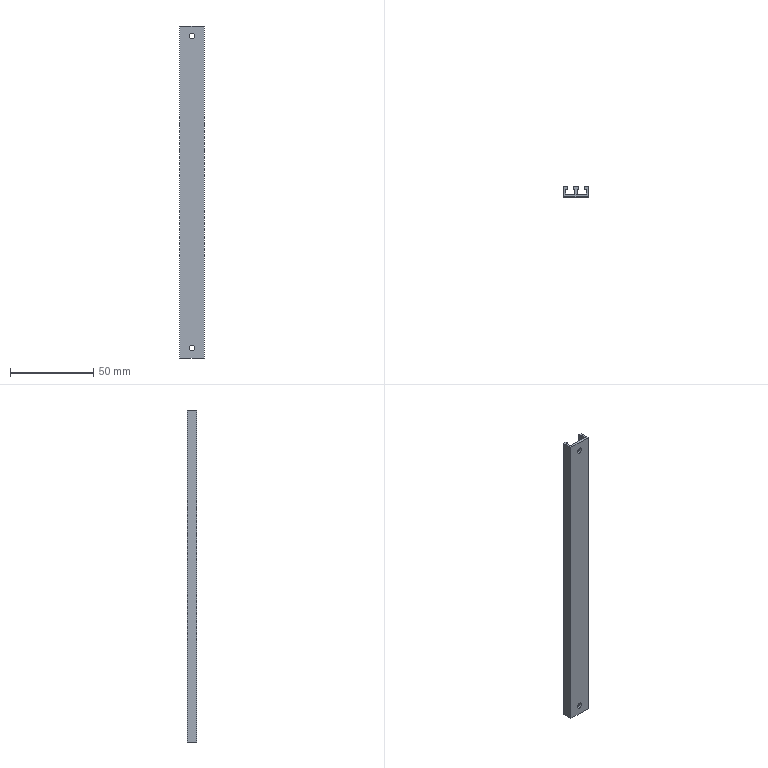Part | STEP file | 10-16 camera shaft sensor mounting strip | 1 solid | 39 faces | box 15 x 6 x 200 mm | volume 9017 mm3 | plane 23 | cylinder 16 | commonest cylinder face diameters 0.4 x12 3.5 x4
STEP:
#1=CARTESIAN_POINT('',(7.5,1.5,-292.25));
#2=VERTEX_POINT('',#1);
#3=CARTESIAN_POINT('',(7.5,1.5,-295.75));
#4=VERTEX_POINT('',#3);
#5=CARTESIAN_POINT('',(7.5,1.5,-294.));
#6=DIRECTION('',(0.,-1.,0.));
#7=DIRECTION('',(1.,0.,0.));
#8=AXIS2_PLACEMENT_3D('',#5,#6,#7);
#9=CIRCLE('',#8,1.75);
#10=EDGE_CURVE('',#2,#4,#9,.T.);
#11=ORIENTED_EDGE('',*,*,#10,.F.);
#12=CARTESIAN_POINT('',(7.5,0.,-292.25));
#13=VERTEX_POINT('',#12);
#14=CARTESIAN_POINT('',(7.5,0.,-292.25));
#15=DIRECTION('',(0.,-1.,0.));
#16=VECTOR('',#15,1000.);
#17=LINE('',#14,#16);
#18=EDGE_CURVE('',#2,#13,#17,.T.);
#19=ORIENTED_EDGE('',*,*,#18,.T.);
#20=CARTESIAN_POINT('',(7.5,0.,-295.75));
#21=VERTEX_POINT('',#20);
#22=CARTESIAN_POINT('',(7.5,0.,-294.));
#23=DIRECTION('',(0.,-1.,0.));
#24=DIRECTION('',(0.,0.,-1.));
#25=AXIS2_PLACEMENT_3D('',#22,#23,#24);
#26=CIRCLE('',#25,1.75);
#27=EDGE_CURVE('',#13,#21,#26,.T.);
#28=ORIENTED_EDGE('',*,*,#27,.T.);
#29=CARTESIAN_POINT('',(7.5,0.,-295.75));
#30=DIRECTION('',(0.,-1.,0.));
#31=VECTOR('',#30,1000.);
#32=LINE('',#29,#31);
#33=EDGE_CURVE('',#4,#21,#32,.T.);
#34=ORIENTED_EDGE('',*,*,#33,.F.);
#35=EDGE_LOOP('',(#11,#19,#28,#34));
#36=FACE_OUTER_BOUND('',#35,.T.);
#37=CARTESIAN_POINT('',(7.5,0.,-294.));
#38=DIRECTION('',(0.,-1.,0.));
#39=DIRECTION('',(0.,0.,-1.));
#40=AXIS2_PLACEMENT_3D('',#37,#38,#39);
#41=CYLINDRICAL_SURFACE('',#40,1.75);
#42=ADVANCED_FACE('',(#36),#41,.F.);
#43=CARTESIAN_POINT('',(7.5,1.5,-104.25));
#44=VERTEX_POINT('',#43);
#45=CARTESIAN_POINT('',(7.5,1.5,-107.75));
#46=VERTEX_POINT('',#45);
#47=CARTESIAN_POINT('',(7.5,1.5,-106.));
#48=DIRECTION('',(0.,-1.,0.));
#49=DIRECTION('',(1.,0.,0.));
#50=AXIS2_PLACEMENT_3D('',#47,#48,#49);
#51=CIRCLE('',#50,1.75);
#52=EDGE_CURVE('',#44,#46,#51,.T.);
#53=ORIENTED_EDGE('',*,*,#52,.F.);
#54=CARTESIAN_POINT('',(7.5,0.,-104.25));
#55=VERTEX_POINT('',#54);
#56=CARTESIAN_POINT('',(7.5,0.,-104.25));
#57=DIRECTION('',(0.,-1.,0.));
#58=VECTOR('',#57,1000.);
#59=LINE('',#56,#58);
#60=EDGE_CURVE('',#44,#55,#59,.T.);
#61=ORIENTED_EDGE('',*,*,#60,.T.);
#62=CARTESIAN_POINT('',(7.5,0.,-107.75));
#63=VERTEX_POINT('',#62);
#64=CARTESIAN_POINT('',(7.5,0.,-106.));
#65=DIRECTION('',(0.,-1.,0.));
#66=DIRECTION('',(0.,0.,-1.));
#67=AXIS2_PLACEMENT_3D('',#64,#65,#66);
#68=CIRCLE('',#67,1.75);
#69=EDGE_CURVE('',#55,#63,#68,.T.);
#70=ORIENTED_EDGE('',*,*,#69,.T.);
#71=CARTESIAN_POINT('',(7.5,0.,-107.75));
#72=DIRECTION('',(0.,-1.,0.));
#73=VECTOR('',#72,1000.);
#74=LINE('',#71,#73);
#75=EDGE_CURVE('',#46,#63,#74,.T.);
#76=ORIENTED_EDGE('',*,*,#75,.F.);
#77=EDGE_LOOP('',(#53,#61,#70,#76));
#78=FACE_OUTER_BOUND('',#77,.T.);
#79=CARTESIAN_POINT('',(7.5,0.,-106.));
#80=DIRECTION('',(0.,-1.,0.));
#81=DIRECTION('',(0.,0.,-1.));
#82=AXIS2_PLACEMENT_3D('',#79,#80,#81);
#83=CYLINDRICAL_SURFACE('',#82,1.75);
#84=ADVANCED_FACE('',(#78),#83,.F.);
#85=CARTESIAN_POINT('',(8.25,4.5,-112.));
#86=VERTEX_POINT('',#85);
#87=CARTESIAN_POINT('',(8.25,4.5,-288.));
#88=VERTEX_POINT('',#87);
#89=CARTESIAN_POINT('',(8.25,4.5,-288.));
#90=DIRECTION('',(0.,0.,-1.));
#91=VECTOR('',#90,1000.);
#92=LINE('',#89,#91);
#93=EDGE_CURVE('',#86,#88,#92,.T.);
#94=ORIENTED_EDGE('',*,*,#93,.F.);
#95=CARTESIAN_POINT('',(8.25,1.5,-112.));
#96=VERTEX_POINT('',#95);
#97=CARTESIAN_POINT('',(8.25,6.,-112.));
#98=DIRECTION('',(0.,-1.,0.));
#99=VECTOR('',#98,1000.);
#100=LINE('',#97,#99);
#101=EDGE_CURVE('',#86,#96,#100,.T.);
#102=ORIENTED_EDGE('',*,*,#101,.T.);
#103=CARTESIAN_POINT('',(8.25,1.5,-288.));
#104=VERTEX_POINT('',#103);
#105=CARTESIAN_POINT('',(8.25,1.5,-288.));
#106=DIRECTION('',(0.,0.,-1.));
#107=VECTOR('',#106,1000.);
#108=LINE('',#105,#107);
#109=EDGE_CURVE('',#96,#104,#108,.T.);
#110=ORIENTED_EDGE('',*,*,#109,.T.);
#111=CARTESIAN_POINT('',(8.25,6.,-288.));
#112=DIRECTION('',(0.,-1.,0.));
#113=VECTOR('',#112,1000.);
#114=LINE('',#111,#113);
#115=EDGE_CURVE('',#88,#104,#114,.T.);
#116=ORIENTED_EDGE('',*,*,#115,.F.);
#117=EDGE_LOOP('',(#94,#102,#110,#116));
#118=FACE_OUTER_BOUND('',#117,.T.);
#119=CARTESIAN_POINT('',(8.25,6.,-288.));
#120=DIRECTION('',(-1.,0.,0.));
#121=DIRECTION('',(0.,-1.,0.));
#122=AXIS2_PLACEMENT_3D('',#119,#120,#121);
#123=PLANE('',#122);
#124=ADVANCED_FACE('',(#118),#123,.F.);
#125=CARTESIAN_POINT('',(6.75,4.5,-288.));
#126=VERTEX_POINT('',#125);
#127=CARTESIAN_POINT('',(6.75,4.5,-112.));
#128=VERTEX_POINT('',#127);
#129=CARTESIAN_POINT('',(6.75,4.5,-112.));
#130=DIRECTION('',(0.,0.,1.));
#131=VECTOR('',#130,1000.);
#132=LINE('',#129,#131);
#133=EDGE_CURVE('',#126,#128,#132,.T.);
#134=ORIENTED_EDGE('',*,*,#133,.F.);
#135=CARTESIAN_POINT('',(6.75,1.5,-288.));
#136=VERTEX_POINT('',#135);
#137=CARTESIAN_POINT('',(6.75,6.,-288.));
#138=DIRECTION('',(0.,-1.,0.));
#139=VECTOR('',#138,1000.);
#140=LINE('',#137,#139);
#141=EDGE_CURVE('',#126,#136,#140,.T.);
#142=ORIENTED_EDGE('',*,*,#141,.T.);
#143=CARTESIAN_POINT('',(6.75,1.5,-112.));
#144=VERTEX_POINT('',#143);
#145=CARTESIAN_POINT('',(6.75,1.5,-112.));
#146=DIRECTION('',(0.,0.,1.));
#147=VECTOR('',#146,1000.);
#148=LINE('',#145,#147);
#149=EDGE_CURVE('',#136,#144,#148,.T.);
#150=ORIENTED_EDGE('',*,*,#149,.T.);
#151=CARTESIAN_POINT('',(6.75,6.,-112.));
#152=DIRECTION('',(0.,-1.,0.));
#153=VECTOR('',#152,1000.);
#154=LINE('',#151,#153);
#155=EDGE_CURVE('',#128,#144,#154,.T.);
#156=ORIENTED_EDGE('',*,*,#155,.F.);
#157=EDGE_LOOP('',(#134,#142,#150,#156));
#158=FACE_OUTER_BOUND('',#157,.T.);
#159=CARTESIAN_POINT('',(6.75,6.,-112.));
#160=DIRECTION('',(1.,0.,0.));
#161=DIRECTION('',(0.,1.,0.));
#162=AXIS2_PLACEMENT_3D('',#159,#160,#161);
#163=PLANE('',#162);
#164=ADVANCED_FACE('',(#158),#163,.F.);
#165=CARTESIAN_POINT('',(7.5,1.5,-294.));
#166=DIRECTION('',(0.,-1.,0.));
#167=DIRECTION('',(1.,0.,0.));
#168=AXIS2_PLACEMENT_3D('',#165,#166,#167);
#169=CIRCLE('',#168,1.75);
#170=EDGE_CURVE('',#4,#2,#169,.T.);
#171=ORIENTED_EDGE('',*,*,#170,.T.);
#172=ORIENTED_EDGE('',*,*,#10,.T.);
#173=EDGE_LOOP('',(#171,#172));
#174=FACE_BOUND('',#173,.T.);
#175=CARTESIAN_POINT('',(7.5,1.5,-106.));
#176=DIRECTION('',(0.,-1.,0.));
#177=DIRECTION('',(1.,0.,0.));
#178=AXIS2_PLACEMENT_3D('',#175,#176,#177);
#179=CIRCLE('',#178,1.75);
#180=EDGE_CURVE('',#46,#44,#179,.T.);
#181=ORIENTED_EDGE('',*,*,#180,.T.);
#182=ORIENTED_EDGE('',*,*,#52,.T.);
#183=EDGE_LOOP('',(#181,#182));
#184=FACE_BOUND('',#183,.T.);
#185=CARTESIAN_POINT('',(1.25,1.5,-100.));
#186=VERTEX_POINT('',#185);
#187=CARTESIAN_POINT('',(13.75,1.5,-100.));
#188=VERTEX_POINT('',#187);
#189=CARTESIAN_POINT('',(1.25,1.5,-100.));
#190=DIRECTION('',(1.,0.,0.));
#191=VECTOR('',#190,1000.);
#192=LINE('',#189,#191);
#193=EDGE_CURVE('',#186,#188,#192,.T.);
#194=ORIENTED_EDGE('',*,*,#193,.T.);
#195=CARTESIAN_POINT('',(13.75,1.5,-300.));
#196=VERTEX_POINT('',#195);
#197=CARTESIAN_POINT('',(13.75,1.5,-300.));
#198=DIRECTION('',(0.,0.,1.));
#199=VECTOR('',#198,1000.);
#200=LINE('',#197,#199);
#201=EDGE_CURVE('',#196,#188,#200,.T.);
#202=ORIENTED_EDGE('',*,*,#201,.F.);
#203=CARTESIAN_POINT('',(1.25,1.5,-300.));
#204=VERTEX_POINT('',#203);
#205=CARTESIAN_POINT('',(1.25,1.5,-300.));
#206=DIRECTION('',(1.,0.,0.));
#207=VECTOR('',#206,1000.);
#208=LINE('',#205,#207);
#209=EDGE_CURVE('',#204,#196,#208,.T.);
#210=ORIENTED_EDGE('',*,*,#209,.F.);
#211=CARTESIAN_POINT('',(1.25,1.5,-300.));
#212=DIRECTION('',(0.,0.,1.));
#213=VECTOR('',#212,1000.);
#214=LINE('',#211,#213);
#215=EDGE_CURVE('',#204,#186,#214,.T.);
#216=ORIENTED_EDGE('',*,*,#215,.T.);
#217=EDGE_LOOP('',(#194,#202,#210,#216));
#218=FACE_OUTER_BOUND('',#217,.T.);
#219=CARTESIAN_POINT('',(6.75,1.5,-288.));
#220=DIRECTION('',(-1.,0.,0.));
#221=VECTOR('',#220,1000.);
#222=LINE('',#219,#221);
#223=EDGE_CURVE('',#104,#136,#222,.T.);
#224=ORIENTED_EDGE('',*,*,#223,.F.);
#225=ORIENTED_EDGE('',*,*,#109,.F.);
#226=CARTESIAN_POINT('',(8.25,1.5,-112.));
#227=DIRECTION('',(1.,0.,0.));
#228=VECTOR('',#227,1000.);
#229=LINE('',#226,#228);
#230=EDGE_CURVE('',#144,#96,#229,.T.);
#231=ORIENTED_EDGE('',*,*,#230,.F.);
#232=ORIENTED_EDGE('',*,*,#149,.F.);
#233=EDGE_LOOP('',(#224,#225,#231,#232));
#234=FACE_BOUND('',#233,.T.);
#235=CARTESIAN_POINT('',(1.25,1.5,-300.));
#236=DIRECTION('',(0.,-1.,0.));
#237=DIRECTION('',(1.,0.,0.));
#238=AXIS2_PLACEMENT_3D('',#235,#236,#237);
#239=PLANE('',#238);
#240=ADVANCED_FACE('',(#174,#184,#218,#234),#239,.F.);
#241=CARTESIAN_POINT('',(12.95,6.,-100.));
#242=VERTEX_POINT('',#241);
#243=CARTESIAN_POINT('',(14.8,6.,-100.));
#244=VERTEX_POINT('',#243);
#245=CARTESIAN_POINT('',(0.,6.,-100.));
#246=DIRECTION('',(1.,0.,0.));
#247=VECTOR('',#246,1000.);
#248=LINE('',#245,#247);
#249=EDGE_CURVE('',#242,#244,#248,.T.);
#250=ORIENTED_EDGE('',*,*,#249,.T.);
#251=CARTESIAN_POINT('',(14.8,6.,-300.));
#252=VERTEX_POINT('',#251);
#253=CARTESIAN_POINT('',(14.8,6.,-100.));
#254=DIRECTION('',(0.,0.,-1.));
#255=VECTOR('',#254,1000.);
#256=LINE('',#253,#255);
#257=EDGE_CURVE('',#244,#252,#256,.T.);
#258=ORIENTED_EDGE('',*,*,#257,.T.);
#259=CARTESIAN_POINT('',(12.95,6.,-300.));
#260=VERTEX_POINT('',#259);
#261=CARTESIAN_POINT('',(15.,6.,-300.));
#262=DIRECTION('',(-1.,0.,0.));
#263=VECTOR('',#262,1000.);
#264=LINE('',#261,#263);
#265=EDGE_CURVE('',#252,#260,#264,.T.);
#266=ORIENTED_EDGE('',*,*,#265,.T.);
#267=CARTESIAN_POINT('',(12.95,6.,-100.));
#268=DIRECTION('',(0.,0.,1.));
#269=VECTOR('',#268,1000.);
#270=LINE('',#267,#269);
#271=EDGE_CURVE('',#260,#242,#270,.T.);
#272=ORIENTED_EDGE('',*,*,#271,.T.);
#273=EDGE_LOOP('',(#250,#258,#266,#272));
#274=FACE_OUTER_BOUND('',#273,.T.);
#275=CARTESIAN_POINT('',(0.,6.,-100.));
#276=DIRECTION('',(0.,1.,0.));
#277=DIRECTION('',(0.,0.,1.));
#278=AXIS2_PLACEMENT_3D('',#275,#276,#277);
#279=PLANE('',#278);
#280=ADVANCED_FACE('',(#274),#279,.T.);
#281=CARTESIAN_POINT('',(0.,0.2,-100.));
#282=VERTEX_POINT('',#281);
#283=CARTESIAN_POINT('',(0.,5.8,-100.));
#284=VERTEX_POINT('',#283);
#285=CARTESIAN_POINT('',(0.,0.,-100.));
#286=DIRECTION('',(0.,1.,0.));
#287=VECTOR('',#286,1000.);
#288=LINE('',#285,#287);
#289=EDGE_CURVE('',#282,#284,#288,.T.);
#290=ORIENTED_EDGE('',*,*,#289,.T.);
#291=CARTESIAN_POINT('',(0.,5.8,-300.));
#292=VERTEX_POINT('',#291);
#293=CARTESIAN_POINT('',(0.,5.8,-300.));
#294=DIRECTION('',(0.,0.,-1.));
#295=VECTOR('',#294,1000.);
#296=LINE('',#293,#295);
#297=EDGE_CURVE('',#284,#292,#296,.T.);
#298=ORIENTED_EDGE('',*,*,#297,.T.);
#299=CARTESIAN_POINT('',(0.,0.2,-300.));
#300=VERTEX_POINT('',#299);
#301=CARTESIAN_POINT('',(0.,0.,-300.));
#302=DIRECTION('',(0.,1.,0.));
#303=VECTOR('',#302,1000.);
#304=LINE('',#301,#303);
#305=EDGE_CURVE('',#300,#292,#304,.T.);
#306=ORIENTED_EDGE('',*,*,#305,.F.);
#307=CARTESIAN_POINT('',(0.,0.2,-100.));
#308=DIRECTION('',(0.,0.,1.));
#309=VECTOR('',#308,1000.);
#310=LINE('',#307,#309);
#311=EDGE_CURVE('',#300,#282,#310,.T.);
#312=ORIENTED_EDGE('',*,*,#311,.T.);
#313=EDGE_LOOP('',(#290,#298,#306,#312));
#314=FACE_OUTER_BOUND('',#313,.T.);
#315=CARTESIAN_POINT('',(0.,0.,-300.));
#316=DIRECTION('',(-1.,0.,0.));
#317=DIRECTION('',(0.,0.,1.));
#318=AXIS2_PLACEMENT_3D('',#315,#316,#317);
#319=PLANE('',#318);
#320=ADVANCED_FACE('',(#314),#319,.T.);
#321=ORIENTED_EDGE('',*,*,#305,.T.);
#322=CARTESIAN_POINT('',(0.2,6.,-300.));
#323=VERTEX_POINT('',#322);
#324=CARTESIAN_POINT('',(0.2,5.8,-300.));
#325=DIRECTION('',(0.,0.,-1.));
#326=DIRECTION('',(-1.,0.,0.));
#327=AXIS2_PLACEMENT_3D('',#324,#325,#326);
#328=CIRCLE('',#327,0.2);
#329=EDGE_CURVE('',#292,#323,#328,.T.);
#330=ORIENTED_EDGE('',*,*,#329,.T.);
#331=CARTESIAN_POINT('',(2.05,6.,-300.));
#332=VERTEX_POINT('',#331);
#333=CARTESIAN_POINT('',(15.,6.,-300.));
#334=DIRECTION('',(-1.,0.,0.));
#335=VECTOR('',#334,1000.);
#336=LINE('',#333,#335);
#337=EDGE_CURVE('',#332,#323,#336,.T.);
#338=ORIENTED_EDGE('',*,*,#337,.F.);
#339=CARTESIAN_POINT('',(2.25,5.8,-300.));
#340=VERTEX_POINT('',#339);
#341=CARTESIAN_POINT('',(2.05,5.8,-300.));
#342=DIRECTION('',(0.,0.,-1.));
#343=DIRECTION('',(-1.,0.,0.));
#344=AXIS2_PLACEMENT_3D('',#341,#342,#343);
#345=CIRCLE('',#344,0.2);
#346=EDGE_CURVE('',#332,#340,#345,.T.);
#347=ORIENTED_EDGE('',*,*,#346,.T.);
#348=CARTESIAN_POINT('',(2.25,4.7,-300.));
#349=VERTEX_POINT('',#348);
#350=CARTESIAN_POINT('',(2.25,6.,-300.));
#351=DIRECTION('',(0.,-1.,0.));
#352=VECTOR('',#351,1000.);
#353=LINE('',#350,#352);
#354=EDGE_CURVE('',#340,#349,#353,.T.);
#355=ORIENTED_EDGE('',*,*,#354,.T.);
#356=CARTESIAN_POINT('',(2.05,4.5,-300.));
#357=VERTEX_POINT('',#356);
#358=CARTESIAN_POINT('',(2.05,4.7,-300.));
#359=DIRECTION('',(0.,0.,-1.));
#360=DIRECTION('',(-1.,0.,0.));
#361=AXIS2_PLACEMENT_3D('',#358,#359,#360);
#362=CIRCLE('',#361,0.2);
#363=EDGE_CURVE('',#349,#357,#362,.T.);
#364=ORIENTED_EDGE('',*,*,#363,.T.);
#365=CARTESIAN_POINT('',(1.25,4.5,-300.));
#366=VERTEX_POINT('',#365);
#367=CARTESIAN_POINT('',(2.25,4.5,-300.));
#368=DIRECTION('',(-1.,0.,0.));
#369=VECTOR('',#368,1000.);
#370=LINE('',#367,#369);
#371=EDGE_CURVE('',#357,#366,#370,.T.);
#372=ORIENTED_EDGE('',*,*,#371,.T.);
#373=CARTESIAN_POINT('',(1.25,4.5,-300.));
#374=DIRECTION('',(0.,-1.,0.));
#375=VECTOR('',#374,1000.);
#376=LINE('',#373,#375);
#377=EDGE_CURVE('',#366,#204,#376,.T.);
#378=ORIENTED_EDGE('',*,*,#377,.T.);
#379=ORIENTED_EDGE('',*,*,#209,.T.);
#380=CARTESIAN_POINT('',(13.75,4.5,-300.));
#381=VERTEX_POINT('',#380);
#382=CARTESIAN_POINT('',(13.75,1.5,-300.));
#383=DIRECTION('',(0.,1.,0.));
#384=VECTOR('',#383,1000.);
#385=LINE('',#382,#384);
#386=EDGE_CURVE('',#196,#381,#385,.T.);
#387=ORIENTED_EDGE('',*,*,#386,.T.);
#388=CARTESIAN_POINT('',(12.95,4.5,-300.));
#389=VERTEX_POINT('',#388);
#390=CARTESIAN_POINT('',(13.75,4.5,-300.));
#391=DIRECTION('',(-1.,0.,0.));
#392=VECTOR('',#391,1000.);
#393=LINE('',#390,#392);
#394=EDGE_CURVE('',#381,#389,#393,.T.);
#395=ORIENTED_EDGE('',*,*,#394,.T.);
#396=CARTESIAN_POINT('',(12.75,4.7,-300.));
#397=VERTEX_POINT('',#396);
#398=CARTESIAN_POINT('',(12.95,4.7,-300.));
#399=DIRECTION('',(0.,0.,-1.));
#400=DIRECTION('',(-1.,0.,0.));
#401=AXIS2_PLACEMENT_3D('',#398,#399,#400);
#402=CIRCLE('',#401,0.2);
#403=EDGE_CURVE('',#389,#397,#402,.T.);
#404=ORIENTED_EDGE('',*,*,#403,.T.);
#405=CARTESIAN_POINT('',(12.75,5.8,-300.));
#406=VERTEX_POINT('',#405);
#407=CARTESIAN_POINT('',(12.75,4.5,-300.));
#408=DIRECTION('',(0.,1.,0.));
#409=VECTOR('',#408,1000.);
#410=LINE('',#407,#409);
#411=EDGE_CURVE('',#397,#406,#410,.T.);
#412=ORIENTED_EDGE('',*,*,#411,.T.);
#413=CARTESIAN_POINT('',(12.95,5.8,-300.));
#414=DIRECTION('',(0.,0.,-1.));
#415=DIRECTION('',(-1.,0.,0.));
#416=AXIS2_PLACEMENT_3D('',#413,#414,#415);
#417=CIRCLE('',#416,0.2);
#418=EDGE_CURVE('',#406,#260,#417,.T.);
#419=ORIENTED_EDGE('',*,*,#418,.T.);
#420=ORIENTED_EDGE('',*,*,#265,.F.);
#421=CARTESIAN_POINT('',(15.,5.8,-300.));
#422=VERTEX_POINT('',#421);
#423=CARTESIAN_POINT('',(14.8,5.8,-300.));
#424=DIRECTION('',(0.,0.,-1.));
#425=DIRECTION('',(-1.,0.,0.));
#426=AXIS2_PLACEMENT_3D('',#423,#424,#425);
#427=CIRCLE('',#426,0.2);
#428=EDGE_CURVE('',#252,#422,#427,.T.);
#429=ORIENTED_EDGE('',*,*,#428,.T.);
#430=CARTESIAN_POINT('',(15.,0.2,-300.));
#431=VERTEX_POINT('',#430);
#432=CARTESIAN_POINT('',(15.,0.,-300.));
#433=DIRECTION('',(0.,1.,0.));
#434=VECTOR('',#433,1000.);
#435=LINE('',#432,#434);
#436=EDGE_CURVE('',#431,#422,#435,.T.);
#437=ORIENTED_EDGE('',*,*,#436,.F.);
#438=CARTESIAN_POINT('',(14.8,0.,-300.));
#439=VERTEX_POINT('',#438);
#440=CARTESIAN_POINT('',(14.8,0.2,-300.));
#441=DIRECTION('',(0.,0.,-1.));
#442=DIRECTION('',(-1.,0.,0.));
#443=AXIS2_PLACEMENT_3D('',#440,#441,#442);
#444=CIRCLE('',#443,0.2);
#445=EDGE_CURVE('',#431,#439,#444,.T.);
#446=ORIENTED_EDGE('',*,*,#445,.T.);
#447=CARTESIAN_POINT('',(0.2,0.,-300.));
#448=VERTEX_POINT('',#447);
#449=CARTESIAN_POINT('',(15.,0.,-300.));
#450=DIRECTION('',(-1.,0.,0.));
#451=VECTOR('',#450,1000.);
#452=LINE('',#449,#451);
#453=EDGE_CURVE('',#439,#448,#452,.T.);
#454=ORIENTED_EDGE('',*,*,#453,.T.);
#455=CARTESIAN_POINT('',(0.2,0.2,-300.));
#456=DIRECTION('',(0.,0.,-1.));
#457=DIRECTION('',(-1.,0.,0.));
#458=AXIS2_PLACEMENT_3D('',#455,#456,#457);
#459=CIRCLE('',#458,0.2);
#460=EDGE_CURVE('',#448,#300,#459,.T.);
#461=ORIENTED_EDGE('',*,*,#460,.T.);
#462=EDGE_LOOP('',(#321,#330,#338,#347,#355,#364,#372,#378,#379,#387,#395,#404,#412,#419,#420,#429,#437,#446,#454,#461));
#463=FACE_OUTER_BOUND('',#462,.T.);
#464=CARTESIAN_POINT('',(15.,0.,-300.));
#465=DIRECTION('',(0.,0.,-1.));
#466=DIRECTION('',(-1.,0.,0.));
#467=AXIS2_PLACEMENT_3D('',#464,#465,#466);
#468=PLANE('',#467);
#469=ADVANCED_FACE('',(#463),#468,.T.);
#470=CARTESIAN_POINT('',(15.,0.2,-100.));
#471=VERTEX_POINT('',#470);
#472=CARTESIAN_POINT('',(15.,5.8,-100.));
#473=VERTEX_POINT('',#472);
#474=CARTESIAN_POINT('',(15.,0.,-100.));
#475=DIRECTION('',(0.,1.,0.));
#476=VECTOR('',#475,1000.);
#477=LINE('',#474,#476);
#478=EDGE_CURVE('',#471,#473,#477,.T.);
#479=ORIENTED_EDGE('',*,*,#478,.F.);
#480=CARTESIAN_POINT('',(15.,0.2,-300.));
#481=DIRECTION('',(0.,0.,-1.));
#482=VECTOR('',#481,1000.);
#483=LINE('',#480,#482);
#484=EDGE_CURVE('',#471,#431,#483,.T.);
#485=ORIENTED_EDGE('',*,*,#484,.T.);
#486=ORIENTED_EDGE('',*,*,#436,.T.);
#487=CARTESIAN_POINT('',(15.,5.8,-100.));
#488=DIRECTION('',(0.,0.,1.));
#489=VECTOR('',#488,1000.);
#490=LINE('',#487,#489);
#491=EDGE_CURVE('',#422,#473,#490,.T.);
#492=ORIENTED_EDGE('',*,*,#491,.T.);
#493=EDGE_LOOP('',(#479,#485,#486,#492));
#494=FACE_OUTER_BOUND('',#493,.T.);
#495=CARTESIAN_POINT('',(15.,0.,-100.));
#496=DIRECTION('',(1.,0.,0.));
#497=DIRECTION('',(0.,0.,-1.));
#498=AXIS2_PLACEMENT_3D('',#495,#496,#497);
#499=PLANE('',#498);
#500=ADVANCED_FACE('',(#494),#499,.T.);
#501=CARTESIAN_POINT('',(0.2,6.,-100.));
#502=VERTEX_POINT('',#501);
#503=CARTESIAN_POINT('',(2.05,6.,-100.));
#504=VERTEX_POINT('',#503);
#505=CARTESIAN_POINT('',(0.,6.,-100.));
#506=DIRECTION('',(1.,0.,0.));
#507=VECTOR('',#506,1000.);
#508=LINE('',#505,#507);
#509=EDGE_CURVE('',#502,#504,#508,.T.);
#510=ORIENTED_EDGE('',*,*,#509,.F.);
#511=CARTESIAN_POINT('',(0.2,5.8,-100.));
#512=DIRECTION('',(0.,0.,1.));
#513=DIRECTION('',(1.,0.,0.));
#514=AXIS2_PLACEMENT_3D('',#511,#512,#513);
#515=CIRCLE('',#514,0.2);
#516=EDGE_CURVE('',#502,#284,#515,.T.);
#517=ORIENTED_EDGE('',*,*,#516,.T.);
#518=ORIENTED_EDGE('',*,*,#289,.F.);
#519=CARTESIAN_POINT('',(0.2,0.,-100.));
#520=VERTEX_POINT('',#519);
#521=CARTESIAN_POINT('',(0.2,0.2,-100.));
#522=DIRECTION('',(0.,0.,1.));
#523=DIRECTION('',(1.,0.,0.));
#524=AXIS2_PLACEMENT_3D('',#521,#522,#523);
#525=CIRCLE('',#524,0.2);
#526=EDGE_CURVE('',#282,#520,#525,.T.);
#527=ORIENTED_EDGE('',*,*,#526,.T.);
#528=CARTESIAN_POINT('',(14.8,0.,-100.));
#529=VERTEX_POINT('',#528);
#530=CARTESIAN_POINT('',(0.,0.,-100.));
#531=DIRECTION('',(1.,0.,0.));
#532=VECTOR('',#531,1000.);
#533=LINE('',#530,#532);
#534=EDGE_CURVE('',#520,#529,#533,.T.);
#535=ORIENTED_EDGE('',*,*,#534,.T.);
#536=CARTESIAN_POINT('',(14.8,0.2,-100.));
#537=DIRECTION('',(0.,0.,1.));
#538=DIRECTION('',(1.,0.,0.));
#539=AXIS2_PLACEMENT_3D('',#536,#537,#538);
#540=CIRCLE('',#539,0.2);
#541=EDGE_CURVE('',#529,#471,#540,.T.);
#542=ORIENTED_EDGE('',*,*,#541,.T.);
#543=ORIENTED_EDGE('',*,*,#478,.T.);
#544=CARTESIAN_POINT('',(14.8,5.8,-100.));
#545=DIRECTION('',(0.,0.,1.));
#546=DIRECTION('',(1.,0.,0.));
#547=AXIS2_PLACEMENT_3D('',#544,#545,#546);
#548=CIRCLE('',#547,0.2);
#549=EDGE_CURVE('',#473,#244,#548,.T.);
#550=ORIENTED_EDGE('',*,*,#549,.T.);
#551=ORIENTED_EDGE('',*,*,#249,.F.);
#552=CARTESIAN_POINT('',(12.75,5.8,-100.));
#553=VERTEX_POINT('',#552);
#554=CARTESIAN_POINT('',(12.95,5.8,-100.));
#555=DIRECTION('',(0.,0.,1.));
#556=DIRECTION('',(1.,0.,0.));
#557=AXIS2_PLACEMENT_3D('',#554,#555,#556);
#558=CIRCLE('',#557,0.2);
#559=EDGE_CURVE('',#242,#553,#558,.T.);
#560=ORIENTED_EDGE('',*,*,#559,.T.);
#561=CARTESIAN_POINT('',(12.75,4.7,-100.));
#562=VERTEX_POINT('',#561);
#563=CARTESIAN_POINT('',(12.75,4.5,-100.));
#564=DIRECTION('',(0.,1.,0.));
#565=VECTOR('',#564,1000.);
#566=LINE('',#563,#565);
#567=EDGE_CURVE('',#562,#553,#566,.T.);
#568=ORIENTED_EDGE('',*,*,#567,.F.);
#569=CARTESIAN_POINT('',(12.95,4.5,-100.));
#570=VERTEX_POINT('',#569);
#571=CARTESIAN_POINT('',(12.95,4.7,-100.));
#572=DIRECTION('',(0.,0.,1.));
#573=DIRECTION('',(1.,0.,0.));
#574=AXIS2_PLACEMENT_3D('',#571,#572,#573);
#575=CIRCLE('',#574,0.2);
#576=EDGE_CURVE('',#562,#570,#575,.T.);
#577=ORIENTED_EDGE('',*,*,#576,.T.);
#578=CARTESIAN_POINT('',(13.75,4.5,-100.));
#579=VERTEX_POINT('',#578);
#580=CARTESIAN_POINT('',(13.75,4.5,-100.));
#581=DIRECTION('',(-1.,0.,0.));
#582=VECTOR('',#581,1000.);
#583=LINE('',#580,#582);
#584=EDGE_CURVE('',#579,#570,#583,.T.);
#585=ORIENTED_EDGE('',*,*,#584,.F.);
#586=CARTESIAN_POINT('',(13.75,1.5,-100.));
#587=DIRECTION('',(0.,1.,0.));
#588=VECTOR('',#587,1000.);
#589=LINE('',#586,#588);
#590=EDGE_CURVE('',#188,#579,#589,.T.);
#591=ORIENTED_EDGE('',*,*,#590,.F.);
#592=ORIENTED_EDGE('',*,*,#193,.F.);
#593=CARTESIAN_POINT('',(1.25,4.5,-100.));
#594=VERTEX_POINT('',#593);
#595=CARTESIAN_POINT('',(1.25,4.5,-100.));
#596=DIRECTION('',(0.,-1.,0.));
#597=VECTOR('',#596,1000.);
#598=LINE('',#595,#597);
#599=EDGE_CURVE('',#594,#186,#598,.T.);
#600=ORIENTED_EDGE('',*,*,#599,.F.);
#601=CARTESIAN_POINT('',(2.05,4.5,-100.));
#602=VERTEX_POINT('',#601);
#603=CARTESIAN_POINT('',(2.25,4.5,-100.));
#604=DIRECTION('',(-1.,0.,0.));
#605=VECTOR('',#604,1000.);
#606=LINE('',#603,#605);
#607=EDGE_CURVE('',#602,#594,#606,.T.);
#608=ORIENTED_EDGE('',*,*,#607,.F.);
#609=CARTESIAN_POINT('',(2.25,4.7,-100.));
#610=VERTEX_POINT('',#609);
#611=CARTESIAN_POINT('',(2.05,4.7,-100.));
#612=DIRECTION('',(0.,0.,1.));
#613=DIRECTION('',(1.,0.,0.));
#614=AXIS2_PLACEMENT_3D('',#611,#612,#613);
#615=CIRCLE('',#614,0.2);
#616=EDGE_CURVE('',#602,#610,#615,.T.);
#617=ORIENTED_EDGE('',*,*,#616,.T.);
#618=CARTESIAN_POINT('',(2.25,5.8,-100.));
#619=VERTEX_POINT('',#618);
#620=CARTESIAN_POINT('',(2.25,6.,-100.));
#621=DIRECTION('',(0.,-1.,0.));
#622=VECTOR('',#621,1000.);
#623=LINE('',#620,#622);
#624=EDGE_CURVE('',#619,#610,#623,.T.);
#625=ORIENTED_EDGE('',*,*,#624,.F.);
#626=CARTESIAN_POINT('',(2.05,5.8,-100.));
#627=DIRECTION('',(0.,0.,1.));
#628=DIRECTION('',(1.,0.,0.));
#629=AXIS2_PLACEMENT_3D('',#626,#627,#628);
#630=CIRCLE('',#629,0.2);
#631=EDGE_CURVE('',#619,#504,#630,.T.);
#632=ORIENTED_EDGE('',*,*,#631,.T.);
#633=EDGE_LOOP('',(#510,#517,#518,#527,#535,#542,#543,#550,#551,#560,#568,#577,#585,#591,#592,#600,#608,#617,#625,#632));
#634=FACE_OUTER_BOUND('',#633,.T.);
#635=CARTESIAN_POINT('',(0.,0.,-100.));
#636=DIRECTION('',(0.,0.,1.));
#637=DIRECTION('',(1.,0.,0.));
#638=AXIS2_PLACEMENT_3D('',#635,#636,#637);
#639=PLANE('',#638);
#640=ADVANCED_FACE('',(#634),#639,.T.);
#641=CARTESIAN_POINT('',(7.5,0.,-294.));
#642=DIRECTION('',(0.,-1.,0.));
#643=DIRECTION('',(0.,0.,-1.));
#644=AXIS2_PLACEMENT_3D('',#641,#642,#643);
#645=CIRCLE('',#644,1.75);
#646=EDGE_CURVE('',#21,#13,#645,.T.);
#647=ORIENTED_EDGE('',*,*,#646,.F.);
#648=ORIENTED_EDGE('',*,*,#27,.F.);
#649=EDGE_LOOP('',(#647,#648));
#650=FACE_BOUND('',#649,.T.);
#651=CARTESIAN_POINT('',(7.5,0.,-106.));
#652=DIRECTION('',(0.,-1.,0.));
#653=DIRECTION('',(0.,0.,-1.));
#654=AXIS2_PLACEMENT_3D('',#651,#652,#653);
#655=CIRCLE('',#654,1.75);
#656=EDGE_CURVE('',#63,#55,#655,.T.);
#657=ORIENTED_EDGE('',*,*,#656,.F.);
#658=ORIENTED_EDGE('',*,*,#69,.F.);
#659=EDGE_LOOP('',(#657,#658));
#660=FACE_BOUND('',#659,.T.);
#661=ORIENTED_EDGE('',*,*,#453,.F.);
#662=CARTESIAN_POINT('',(14.8,0.,-100.));
#663=DIRECTION('',(0.,0.,1.));
#664=VECTOR('',#663,1000.);
#665=LINE('',#662,#664);
#666=EDGE_CURVE('',#439,#529,#665,.T.);
#667=ORIENTED_EDGE('',*,*,#666,.T.);
#668=ORIENTED_EDGE('',*,*,#534,.F.);
#669=CARTESIAN_POINT('',(0.2,0.,-300.));
#670=DIRECTION('',(0.,0.,-1.));
#671=VECTOR('',#670,1000.);
#672=LINE('',#669,#671);
#673=EDGE_CURVE('',#520,#448,#672,.T.);
#674=ORIENTED_EDGE('',*,*,#673,.T.);
#675=EDGE_LOOP('',(#661,#667,#668,#674));
#676=FACE_OUTER_BOUND('',#675,.T.);
#677=CARTESIAN_POINT('',(0.,0.,-100.));
#678=DIRECTION('',(0.,1.,0.));
#679=DIRECTION('',(0.,0.,1.));
#680=AXIS2_PLACEMENT_3D('',#677,#678,#679);
#681=PLANE('',#680);
#682=ADVANCED_FACE('',(#650,#660,#676),#681,.F.);
#683=ORIENTED_EDGE('',*,*,#337,.T.);
#684=CARTESIAN_POINT('',(0.2,6.,-100.));
#685=DIRECTION('',(0.,0.,1.));
#686=VECTOR('',#685,1000.);
#687=LINE('',#684,#686);
#688=EDGE_CURVE('',#323,#502,#687,.T.);
#689=ORIENTED_EDGE('',*,*,#688,.T.);
#690=ORIENTED_EDGE('',*,*,#509,.T.);
#691=CARTESIAN_POINT('',(2.05,6.,-300.));
#692=DIRECTION('',(0.,0.,-1.));
#693=VECTOR('',#692,1000.);
#694=LINE('',#691,#693);
#695=EDGE_CURVE('',#504,#332,#694,.T.);
#696=ORIENTED_EDGE('',*,*,#695,.T.);
#697=EDGE_LOOP('',(#683,#689,#690,#696));
#698=FACE_OUTER_BOUND('',#697,.T.);
#699=CARTESIAN_POINT('',(0.,6.,-100.));
#700=DIRECTION('',(0.,1.,0.));
#701=DIRECTION('',(0.,0.,1.));
#702=AXIS2_PLACEMENT_3D('',#699,#700,#701);
#703=PLANE('',#702);
#704=ADVANCED_FACE('',(#698),#703,.T.);
#705=ORIENTED_EDGE('',*,*,#567,.T.);
#706=CARTESIAN_POINT('',(12.75,5.8,-300.));
#707=DIRECTION('',(0.,0.,-1.));
#708=VECTOR('',#707,1000.);
#709=LINE('',#706,#708);
#710=EDGE_CURVE('',#553,#406,#709,.T.);
#711=ORIENTED_EDGE('',*,*,#710,.T.);
#712=ORIENTED_EDGE('',*,*,#411,.F.);
#713=CARTESIAN_POINT('',(12.75,4.7,-300.));
#714=DIRECTION('',(0.,0.,1.));
#715=VECTOR('',#714,1000.);
#716=LINE('',#713,#715);
#717=EDGE_CURVE('',#397,#562,#716,.T.);
#718=ORIENTED_EDGE('',*,*,#717,.T.);
#719=EDGE_LOOP('',(#705,#711,#712,#718));
#720=FACE_OUTER_BOUND('',#719,.T.);
#721=CARTESIAN_POINT('',(12.75,4.5,-300.));
#722=DIRECTION('',(1.,0.,0.));
#723=DIRECTION('',(0.,1.,0.));
#724=AXIS2_PLACEMENT_3D('',#721,#722,#723);
#725=PLANE('',#724);
#726=ADVANCED_FACE('',(#720),#725,.F.);
#727=ORIENTED_EDGE('',*,*,#584,.T.);
#728=CARTESIAN_POINT('',(12.95,4.5,-300.));
#729=DIRECTION('',(0.,0.,-1.));
#730=VECTOR('',#729,1000.);
#731=LINE('',#728,#730);
#732=EDGE_CURVE('',#570,#389,#731,.T.);
#733=ORIENTED_EDGE('',*,*,#732,.T.);
#734=ORIENTED_EDGE('',*,*,#394,.F.);
#735=CARTESIAN_POINT('',(13.75,4.5,-300.));
#736=DIRECTION('',(0.,0.,1.));
#737=VECTOR('',#736,1000.);
#738=LINE('',#735,#737);
#739=EDGE_CURVE('',#381,#579,#738,.T.);
#740=ORIENTED_EDGE('',*,*,#739,.T.);
#741=EDGE_LOOP('',(#727,#733,#734,#740));
#742=FACE_OUTER_BOUND('',#741,.T.);
#743=CARTESIAN_POINT('',(13.75,4.5,-300.));
#744=DIRECTION('',(0.,1.,0.));
#745=DIRECTION('',(-1.,0.,0.));
#746=AXIS2_PLACEMENT_3D('',#743,#744,#745);
#747=PLANE('',#746);
#748=ADVANCED_FACE('',(#742),#747,.F.);
#749=ORIENTED_EDGE('',*,*,#590,.T.);
#750=ORIENTED_EDGE('',*,*,#739,.F.);
#751=ORIENTED_EDGE('',*,*,#386,.F.);
#752=ORIENTED_EDGE('',*,*,#201,.T.);
#753=EDGE_LOOP('',(#749,#750,#751,#752));
#754=FACE_OUTER_BOUND('',#753,.T.);
#755=CARTESIAN_POINT('',(13.75,1.5,-300.));
#756=DIRECTION('',(1.,0.,0.));
#757=DIRECTION('',(0.,0.,-1.));
#758=AXIS2_PLACEMENT_3D('',#755,#756,#757);
#759=PLANE('',#758);
#760=ADVANCED_FACE('',(#754),#759,.F.);
#761=ORIENTED_EDGE('',*,*,#599,.T.);
#762=ORIENTED_EDGE('',*,*,#215,.F.);
#763=ORIENTED_EDGE('',*,*,#377,.F.);
#764=CARTESIAN_POINT('',(1.25,4.5,-300.));
#765=DIRECTION('',(0.,0.,1.));
#766=VECTOR('',#765,1000.);
#767=LINE('',#764,#766);
#768=EDGE_CURVE('',#366,#594,#767,.T.);
#769=ORIENTED_EDGE('',*,*,#768,.T.);
#770=EDGE_LOOP('',(#761,#762,#763,#769));
#771=FACE_OUTER_BOUND('',#770,.T.);
#772=CARTESIAN_POINT('',(1.25,4.5,-300.));
#773=DIRECTION('',(-1.,0.,0.));
#774=DIRECTION('',(0.,0.,1.));
#775=AXIS2_PLACEMENT_3D('',#772,#773,#774);
#776=PLANE('',#775);
#777=ADVANCED_FACE('',(#771),#776,.F.);
#778=ORIENTED_EDGE('',*,*,#371,.F.);
#779=CARTESIAN_POINT('',(2.05,4.5,-300.));
#780=DIRECTION('',(0.,0.,1.));
#781=VECTOR('',#780,1000.);
#782=LINE('',#779,#781);
#783=EDGE_CURVE('',#357,#602,#782,.T.);
#784=ORIENTED_EDGE('',*,*,#783,.T.);
#785=ORIENTED_EDGE('',*,*,#607,.T.);
#786=ORIENTED_EDGE('',*,*,#768,.F.);
#787=EDGE_LOOP('',(#778,#784,#785,#786));
#788=FACE_OUTER_BOUND('',#787,.T.);
#789=CARTESIAN_POINT('',(2.25,4.5,-300.));
#790=DIRECTION('',(0.,1.,0.));
#791=DIRECTION('',(0.,0.,1.));
#792=AXIS2_PLACEMENT_3D('',#789,#790,#791);
#793=PLANE('',#792);
#794=ADVANCED_FACE('',(#788),#793,.F.);
#795=ORIENTED_EDGE('',*,*,#354,.F.);
#796=CARTESIAN_POINT('',(2.25,5.8,-100.));
#797=DIRECTION('',(0.,0.,1.));
#798=VECTOR('',#797,1000.);
#799=LINE('',#796,#798);
#800=EDGE_CURVE('',#340,#619,#799,.T.);
#801=ORIENTED_EDGE('',*,*,#800,.T.);
#802=ORIENTED_EDGE('',*,*,#624,.T.);
#803=CARTESIAN_POINT('',(2.25,4.7,-300.));
#804=DIRECTION('',(0.,0.,-1.));
#805=VECTOR('',#804,1000.);
#806=LINE('',#803,#805);
#807=EDGE_CURVE('',#610,#349,#806,.T.);
#808=ORIENTED_EDGE('',*,*,#807,.T.);
#809=EDGE_LOOP('',(#795,#801,#802,#808));
#810=FACE_OUTER_BOUND('',#809,.T.);
#811=CARTESIAN_POINT('',(2.25,6.,-300.));
#812=DIRECTION('',(-1.,0.,0.));
#813=DIRECTION('',(0.,0.,1.));
#814=AXIS2_PLACEMENT_3D('',#811,#812,#813);
#815=PLANE('',#814);
#816=ADVANCED_FACE('',(#810),#815,.F.);
#817=CARTESIAN_POINT('',(9.05,6.,-288.));
#818=VERTEX_POINT('',#817);
#819=CARTESIAN_POINT('',(5.95,6.,-288.));
#820=VERTEX_POINT('',#819);
#821=CARTESIAN_POINT('',(6.75,6.,-288.));
#822=DIRECTION('',(-1.,0.,0.));
#823=VECTOR('',#822,1000.);
#824=LINE('',#821,#823);
#825=EDGE_CURVE('',#818,#820,#824,.T.);
#826=ORIENTED_EDGE('',*,*,#825,.F.);
#827=CARTESIAN_POINT('',(9.25,5.8,-288.));
#828=VERTEX_POINT('',#827);
#829=CARTESIAN_POINT('',(9.05,5.8,-288.));
#830=DIRECTION('',(0.,0.,-1.));
#831=DIRECTION('',(1.,0.,0.));
#832=AXIS2_PLACEMENT_3D('',#829,#830,#831);
#833=CIRCLE('',#832,0.2);
#834=EDGE_CURVE('',#818,#828,#833,.T.);
#835=ORIENTED_EDGE('',*,*,#834,.T.);
#836=CARTESIAN_POINT('',(9.25,4.7,-288.));
#837=VERTEX_POINT('',#836);
#838=CARTESIAN_POINT('',(9.25,6.,-288.));
#839=DIRECTION('',(0.,1.,0.));
#840=VECTOR('',#839,1000.);
#841=LINE('',#838,#840);
#842=EDGE_CURVE('',#837,#828,#841,.T.);
#843=ORIENTED_EDGE('',*,*,#842,.F.);
#844=CARTESIAN_POINT('',(9.05,4.5,-288.));
#845=VERTEX_POINT('',#844);
#846=CARTESIAN_POINT('',(9.05,4.7,-288.));
#847=DIRECTION('',(0.,0.,-1.));
#848=DIRECTION('',(1.,0.,0.));
#849=AXIS2_PLACEMENT_3D('',#846,#847,#848);
#850=CIRCLE('',#849,0.2);
#851=EDGE_CURVE('',#837,#845,#850,.T.);
#852=ORIENTED_EDGE('',*,*,#851,.T.);
#853=CARTESIAN_POINT('',(9.25,4.5,-288.));
#854=DIRECTION('',(-1.,0.,0.));
#855=VECTOR('',#854,1000.);
#856=LINE('',#853,#855);
#857=EDGE_CURVE('',#845,#88,#856,.T.);
#858=ORIENTED_EDGE('',*,*,#857,.T.);
#859=ORIENTED_EDGE('',*,*,#115,.T.);
#860=ORIENTED_EDGE('',*,*,#223,.T.);
#861=ORIENTED_EDGE('',*,*,#141,.F.);
#862=CARTESIAN_POINT('',(5.95,4.5,-288.));
#863=VERTEX_POINT('',#862);
#864=CARTESIAN_POINT('',(5.75,4.5,-288.));
#865=DIRECTION('',(1.,0.,0.));
#866=VECTOR('',#865,1000.);
#867=LINE('',#864,#866);
#868=EDGE_CURVE('',#863,#126,#867,.T.);
#869=ORIENTED_EDGE('',*,*,#868,.F.);
#870=CARTESIAN_POINT('',(5.75,4.7,-288.));
#871=VERTEX_POINT('',#870);
#872=CARTESIAN_POINT('',(5.95,4.7,-288.));
#873=DIRECTION('',(0.,0.,-1.));
#874=DIRECTION('',(1.,0.,0.));
#875=AXIS2_PLACEMENT_3D('',#872,#873,#874);
#876=CIRCLE('',#875,0.2);
#877=EDGE_CURVE('',#863,#871,#876,.T.);
#878=ORIENTED_EDGE('',*,*,#877,.T.);
#879=CARTESIAN_POINT('',(5.75,5.8,-288.));
#880=VERTEX_POINT('',#879);
#881=CARTESIAN_POINT('',(5.75,4.5,-288.));
#882=DIRECTION('',(0.,-1.,0.));
#883=VECTOR('',#882,1000.);
#884=LINE('',#881,#883);
#885=EDGE_CURVE('',#880,#871,#884,.T.);
#886=ORIENTED_EDGE('',*,*,#885,.F.);
#887=CARTESIAN_POINT('',(5.95,5.8,-288.));
#888=DIRECTION('',(0.,0.,-1.));
#889=DIRECTION('',(1.,0.,0.));
#890=AXIS2_PLACEMENT_3D('',#887,#888,#889);
#891=CIRCLE('',#890,0.2);
#892=EDGE_CURVE('',#880,#820,#891,.T.);
#893=ORIENTED_EDGE('',*,*,#892,.T.);
#894=EDGE_LOOP('',(#826,#835,#843,#852,#858,#859,#860,#861,#869,#878,#886,#893));
#895=FACE_OUTER_BOUND('',#894,.T.);
#896=CARTESIAN_POINT('',(6.75,6.,-288.));
#897=DIRECTION('',(0.,0.,1.));
#898=DIRECTION('',(1.,0.,0.));
#899=AXIS2_PLACEMENT_3D('',#896,#897,#898);
#900=PLANE('',#899);
#901=ADVANCED_FACE('',(#895),#900,.F.);
#902=CARTESIAN_POINT('',(9.25,5.8,-112.));
#903=VERTEX_POINT('',#902);
#904=CARTESIAN_POINT('',(9.25,4.7,-112.));
#905=VERTEX_POINT('',#904);
#906=CARTESIAN_POINT('',(9.25,4.5,-112.));
#907=DIRECTION('',(0.,-1.,0.));
#908=VECTOR('',#907,1000.);
#909=LINE('',#906,#908);
#910=EDGE_CURVE('',#903,#905,#909,.T.);
#911=ORIENTED_EDGE('',*,*,#910,.F.);
#912=CARTESIAN_POINT('',(9.05,6.,-112.));
#913=VERTEX_POINT('',#912);
#914=CARTESIAN_POINT('',(9.05,5.8,-112.));
#915=DIRECTION('',(0.,0.,1.));
#916=DIRECTION('',(-1.,0.,0.));
#917=AXIS2_PLACEMENT_3D('',#914,#915,#916);
#918=CIRCLE('',#917,0.2);
#919=EDGE_CURVE('',#903,#913,#918,.T.);
#920=ORIENTED_EDGE('',*,*,#919,.T.);
#921=CARTESIAN_POINT('',(5.95,6.,-112.));
#922=VERTEX_POINT('',#921);
#923=CARTESIAN_POINT('',(8.25,6.,-112.));
#924=DIRECTION('',(1.,0.,0.));
#925=VECTOR('',#924,1000.);
#926=LINE('',#923,#925);
#927=EDGE_CURVE('',#922,#913,#926,.T.);
#928=ORIENTED_EDGE('',*,*,#927,.F.);
#929=CARTESIAN_POINT('',(5.75,5.8,-112.));
#930=VERTEX_POINT('',#929);
#931=CARTESIAN_POINT('',(5.95,5.8,-112.));
#932=DIRECTION('',(0.,0.,1.));
#933=DIRECTION('',(-1.,0.,0.));
#934=AXIS2_PLACEMENT_3D('',#931,#932,#933);
#935=CIRCLE('',#934,0.2);
#936=EDGE_CURVE('',#922,#930,#935,.T.);
#937=ORIENTED_EDGE('',*,*,#936,.T.);
#938=CARTESIAN_POINT('',(5.75,4.7,-112.));
#939=VERTEX_POINT('',#938);
#940=CARTESIAN_POINT('',(5.75,6.,-112.));
#941=DIRECTION('',(0.,1.,0.));
#942=VECTOR('',#941,1000.);
#943=LINE('',#940,#942);
#944=EDGE_CURVE('',#939,#930,#943,.T.);
#945=ORIENTED_EDGE('',*,*,#944,.F.);
#946=CARTESIAN_POINT('',(5.95,4.5,-112.));
#947=VERTEX_POINT('',#946);
#948=CARTESIAN_POINT('',(5.95,4.7,-112.));
#949=DIRECTION('',(0.,0.,1.));
#950=DIRECTION('',(-1.,0.,0.));
#951=AXIS2_PLACEMENT_3D('',#948,#949,#950);
#952=CIRCLE('',#951,0.2);
#953=EDGE_CURVE('',#939,#947,#952,.T.);
#954=ORIENTED_EDGE('',*,*,#953,.T.);
#955=CARTESIAN_POINT('',(5.75,4.5,-112.));
#956=DIRECTION('',(1.,0.,0.));
#957=VECTOR('',#956,1000.);
#958=LINE('',#955,#957);
#959=EDGE_CURVE('',#947,#128,#958,.T.);
#960=ORIENTED_EDGE('',*,*,#959,.T.);
#961=ORIENTED_EDGE('',*,*,#155,.T.);
#962=ORIENTED_EDGE('',*,*,#230,.T.);
#963=ORIENTED_EDGE('',*,*,#101,.F.);
#964=CARTESIAN_POINT('',(9.05,4.5,-112.));
#965=VERTEX_POINT('',#964);
#966=CARTESIAN_POINT('',(9.25,4.5,-112.));
#967=DIRECTION('',(-1.,0.,0.));
#968=VECTOR('',#967,1000.);
#969=LINE('',#966,#968);
#970=EDGE_CURVE('',#965,#86,#969,.T.);
#971=ORIENTED_EDGE('',*,*,#970,.F.);
#972=CARTESIAN_POINT('',(9.05,4.7,-112.));
#973=DIRECTION('',(0.,0.,1.));
#974=DIRECTION('',(-1.,0.,0.));
#975=AXIS2_PLACEMENT_3D('',#972,#973,#974);
#976=CIRCLE('',#975,0.2);
#977=EDGE_CURVE('',#965,#905,#976,.T.);
#978=ORIENTED_EDGE('',*,*,#977,.T.);
#979=EDGE_LOOP('',(#911,#920,#928,#937,#945,#954,#960,#961,#962,#963,#971,#978));
#980=FACE_OUTER_BOUND('',#979,.T.);
#981=CARTESIAN_POINT('',(8.25,6.,-112.));
#982=DIRECTION('',(0.,0.,-1.));
#983=DIRECTION('',(-1.,0.,0.));
#984=AXIS2_PLACEMENT_3D('',#981,#982,#983);
#985=PLANE('',#984);
#986=ADVANCED_FACE('',(#980),#985,.F.);
#987=ORIENTED_EDGE('',*,*,#927,.T.);
#988=CARTESIAN_POINT('',(9.05,6.,-288.));
#989=DIRECTION('',(0.,0.,-1.));
#990=VECTOR('',#989,1000.);
#991=LINE('',#988,#990);
#992=EDGE_CURVE('',#913,#818,#991,.T.);
#993=ORIENTED_EDGE('',*,*,#992,.T.);
#994=ORIENTED_EDGE('',*,*,#825,.T.);
#995=CARTESIAN_POINT('',(5.95,6.,-288.));
#996=DIRECTION('',(0.,0.,1.));
#997=VECTOR('',#996,1000.);
#998=LINE('',#995,#997);
#999=EDGE_CURVE('',#820,#922,#998,.T.);
#1000=ORIENTED_EDGE('',*,*,#999,.T.);
#1001=EDGE_LOOP('',(#987,#993,#994,#1000));
#1002=FACE_OUTER_BOUND('',#1001,.T.);
#1003=CARTESIAN_POINT('',(8.25,6.,-288.));
#1004=DIRECTION('',(0.,-1.,0.));
#1005=DIRECTION('',(1.,0.,0.));
#1006=AXIS2_PLACEMENT_3D('',#1003,#1004,#1005);
#1007=PLANE('',#1006);
#1008=ADVANCED_FACE('',(#1002),#1007,.F.);
#1009=ORIENTED_EDGE('',*,*,#959,.F.);
#1010=CARTESIAN_POINT('',(5.95,4.5,-112.));
#1011=DIRECTION('',(0.,0.,-1.));
#1012=VECTOR('',#1011,1000.);
#1013=LINE('',#1010,#1012);
#1014=EDGE_CURVE('',#947,#863,#1013,.T.);
#1015=ORIENTED_EDGE('',*,*,#1014,.T.);
#1016=ORIENTED_EDGE('',*,*,#868,.T.);
#1017=ORIENTED_EDGE('',*,*,#133,.T.);
#1018=EDGE_LOOP('',(#1009,#1015,#1016,#1017));
#1019=FACE_OUTER_BOUND('',#1018,.T.);
#1020=CARTESIAN_POINT('',(5.75,4.5,-112.));
#1021=DIRECTION('',(0.,1.,0.));
#1022=DIRECTION('',(-1.,0.,0.));
#1023=AXIS2_PLACEMENT_3D('',#1020,#1021,#1022);
#1024=PLANE('',#1023);
#1025=ADVANCED_FACE('',(#1019),#1024,.F.);
#1026=ORIENTED_EDGE('',*,*,#885,.T.);
#1027=CARTESIAN_POINT('',(5.75,4.7,-112.));
#1028=DIRECTION('',(0.,0.,1.));
#1029=VECTOR('',#1028,1000.);
#1030=LINE('',#1027,#1029);
#1031=EDGE_CURVE('',#871,#939,#1030,.T.);
#1032=ORIENTED_EDGE('',*,*,#1031,.T.);
#1033=ORIENTED_EDGE('',*,*,#944,.T.);
#1034=CARTESIAN_POINT('',(5.75,5.8,-112.));
#1035=DIRECTION('',(0.,0.,-1.));
#1036=VECTOR('',#1035,1000.);
#1037=LINE('',#1034,#1036);
#1038=EDGE_CURVE('',#930,#880,#1037,.T.);
#1039=ORIENTED_EDGE('',*,*,#1038,.T.);
#1040=EDGE_LOOP('',(#1026,#1032,#1033,#1039));
#1041=FACE_OUTER_BOUND('',#1040,.T.);
#1042=CARTESIAN_POINT('',(5.75,6.,-112.));
#1043=DIRECTION('',(1.,0.,0.));
#1044=DIRECTION('',(0.,1.,0.));
#1045=AXIS2_PLACEMENT_3D('',#1042,#1043,#1044);
#1046=PLANE('',#1045);
#1047=ADVANCED_FACE('',(#1041),#1046,.F.);
#1048=ORIENTED_EDGE('',*,*,#857,.F.);
#1049=CARTESIAN_POINT('',(9.05,4.5,-288.));
#1050=DIRECTION('',(0.,0.,1.));
#1051=VECTOR('',#1050,1000.);
#1052=LINE('',#1049,#1051);
#1053=EDGE_CURVE('',#845,#965,#1052,.T.);
#1054=ORIENTED_EDGE('',*,*,#1053,.T.);
#1055=ORIENTED_EDGE('',*,*,#970,.T.);
#1056=ORIENTED_EDGE('',*,*,#93,.T.);
#1057=EDGE_LOOP('',(#1048,#1054,#1055,#1056));
#1058=FACE_OUTER_BOUND('',#1057,.T.);
#1059=CARTESIAN_POINT('',(9.25,4.5,-288.));
#1060=DIRECTION('',(0.,1.,0.));
#1061=DIRECTION('',(-1.,0.,0.));
#1062=AXIS2_PLACEMENT_3D('',#1059,#1060,#1061);
#1063=PLANE('',#1062);
#1064=ADVANCED_FACE('',(#1058),#1063,.F.);
#1065=ORIENTED_EDGE('',*,*,#842,.T.);
#1066=CARTESIAN_POINT('',(9.25,5.8,-112.));
#1067=DIRECTION('',(0.,0.,1.));
#1068=VECTOR('',#1067,1000.);
#1069=LINE('',#1066,#1068);
#1070=EDGE_CURVE('',#828,#903,#1069,.T.);
#1071=ORIENTED_EDGE('',*,*,#1070,.T.);
#1072=ORIENTED_EDGE('',*,*,#910,.T.);
#1073=CARTESIAN_POINT('',(9.25,4.7,-112.));
#1074=DIRECTION('',(0.,0.,-1.));
#1075=VECTOR('',#1074,1000.);
#1076=LINE('',#1073,#1075);
#1077=EDGE_CURVE('',#905,#837,#1076,.T.);
#1078=ORIENTED_EDGE('',*,*,#1077,.T.);
#1079=EDGE_LOOP('',(#1065,#1071,#1072,#1078));
#1080=FACE_OUTER_BOUND('',#1079,.T.);
#1081=CARTESIAN_POINT('',(9.25,4.5,-112.));
#1082=DIRECTION('',(-1.,0.,0.));
#1083=DIRECTION('',(0.,-1.,0.));
#1084=AXIS2_PLACEMENT_3D('',#1081,#1082,#1083);
#1085=PLANE('',#1084);
#1086=ADVANCED_FACE('',(#1080),#1085,.F.);
#1087=ORIENTED_EDGE('',*,*,#60,.F.);
#1088=ORIENTED_EDGE('',*,*,#180,.F.);
#1089=ORIENTED_EDGE('',*,*,#75,.T.);
#1090=ORIENTED_EDGE('',*,*,#656,.T.);
#1091=EDGE_LOOP('',(#1087,#1088,#1089,#1090));
#1092=FACE_OUTER_BOUND('',#1091,.T.);
#1093=CARTESIAN_POINT('',(7.5,0.,-106.));
#1094=DIRECTION('',(0.,-1.,0.));
#1095=DIRECTION('',(0.,0.,-1.));
#1096=AXIS2_PLACEMENT_3D('',#1093,#1094,#1095);
#1097=CYLINDRICAL_SURFACE('',#1096,1.75);
#1098=ADVANCED_FACE('',(#1092),#1097,.F.);
#1099=ORIENTED_EDGE('',*,*,#18,.F.);
#1100=ORIENTED_EDGE('',*,*,#170,.F.);
#1101=ORIENTED_EDGE('',*,*,#33,.T.);
#1102=ORIENTED_EDGE('',*,*,#646,.T.);
#1103=EDGE_LOOP('',(#1099,#1100,#1101,#1102));
#1104=FACE_OUTER_BOUND('',#1103,.T.);
#1105=CARTESIAN_POINT('',(7.5,0.,-294.));
#1106=DIRECTION('',(0.,-1.,0.));
#1107=DIRECTION('',(0.,0.,-1.));
#1108=AXIS2_PLACEMENT_3D('',#1105,#1106,#1107);
#1109=CYLINDRICAL_SURFACE('',#1108,1.75);
#1110=ADVANCED_FACE('',(#1104),#1109,.F.);
#1111=ORIENTED_EDGE('',*,*,#329,.F.);
#1112=ORIENTED_EDGE('',*,*,#297,.F.);
#1113=ORIENTED_EDGE('',*,*,#516,.F.);
#1114=ORIENTED_EDGE('',*,*,#688,.F.);
#1115=EDGE_LOOP('',(#1111,#1112,#1113,#1114));
#1116=FACE_OUTER_BOUND('',#1115,.T.);
#1117=CARTESIAN_POINT('',(0.2,5.8,-100.));
#1118=DIRECTION('',(0.,0.,1.));
#1119=DIRECTION('',(1.,0.,0.));
#1120=AXIS2_PLACEMENT_3D('',#1117,#1118,#1119);
#1121=CYLINDRICAL_SURFACE('',#1120,0.2);
#1122=ADVANCED_FACE('',(#1116),#1121,.T.);
#1123=ORIENTED_EDGE('',*,*,#541,.F.);
#1124=ORIENTED_EDGE('',*,*,#666,.F.);
#1125=ORIENTED_EDGE('',*,*,#445,.F.);
#1126=ORIENTED_EDGE('',*,*,#484,.F.);
#1127=EDGE_LOOP('',(#1123,#1124,#1125,#1126));
#1128=FACE_OUTER_BOUND('',#1127,.T.);
#1129=CARTESIAN_POINT('',(14.8,0.2,-100.));
#1130=DIRECTION('',(0.,0.,1.));
#1131=DIRECTION('',(1.,0.,0.));
#1132=AXIS2_PLACEMENT_3D('',#1129,#1130,#1131);
#1133=CYLINDRICAL_SURFACE('',#1132,0.2);
#1134=ADVANCED_FACE('',(#1128),#1133,.T.);
#1135=ORIENTED_EDGE('',*,*,#549,.F.);
#1136=ORIENTED_EDGE('',*,*,#491,.F.);
#1137=ORIENTED_EDGE('',*,*,#428,.F.);
#1138=ORIENTED_EDGE('',*,*,#257,.F.);
#1139=EDGE_LOOP('',(#1135,#1136,#1137,#1138));
#1140=FACE_OUTER_BOUND('',#1139,.T.);
#1141=CARTESIAN_POINT('',(14.8,5.8,-100.));
#1142=DIRECTION('',(0.,0.,-1.));
#1143=DIRECTION('',(-1.,0.,0.));
#1144=AXIS2_PLACEMENT_3D('',#1141,#1142,#1143);
#1145=CYLINDRICAL_SURFACE('',#1144,0.2);
#1146=ADVANCED_FACE('',(#1140),#1145,.T.);
#1147=ORIENTED_EDGE('',*,*,#834,.F.);
#1148=ORIENTED_EDGE('',*,*,#992,.F.);
#1149=ORIENTED_EDGE('',*,*,#919,.F.);
#1150=ORIENTED_EDGE('',*,*,#1070,.F.);
#1151=EDGE_LOOP('',(#1147,#1148,#1149,#1150));
#1152=FACE_OUTER_BOUND('',#1151,.T.);
#1153=CARTESIAN_POINT('',(9.05,5.8,-112.));
#1154=DIRECTION('',(0.,0.,1.));
#1155=DIRECTION('',(1.,0.,0.));
#1156=AXIS2_PLACEMENT_3D('',#1153,#1154,#1155);
#1157=CYLINDRICAL_SURFACE('',#1156,0.2);
#1158=ADVANCED_FACE('',(#1152),#1157,.T.);
#1159=ORIENTED_EDGE('',*,*,#346,.F.);
#1160=ORIENTED_EDGE('',*,*,#695,.F.);
#1161=ORIENTED_EDGE('',*,*,#631,.F.);
#1162=ORIENTED_EDGE('',*,*,#800,.F.);
#1163=EDGE_LOOP('',(#1159,#1160,#1161,#1162));
#1164=FACE_OUTER_BOUND('',#1163,.T.);
#1165=CARTESIAN_POINT('',(2.05,5.8,-300.));
#1166=DIRECTION('',(0.,0.,-1.));
#1167=DIRECTION('',(-1.,0.,0.));
#1168=AXIS2_PLACEMENT_3D('',#1165,#1166,#1167);
#1169=CYLINDRICAL_SURFACE('',#1168,0.2);
#1170=ADVANCED_FACE('',(#1164),#1169,.T.);
#1171=ORIENTED_EDGE('',*,*,#877,.F.);
#1172=ORIENTED_EDGE('',*,*,#1014,.F.);
#1173=ORIENTED_EDGE('',*,*,#953,.F.);
#1174=ORIENTED_EDGE('',*,*,#1031,.F.);
#1175=EDGE_LOOP('',(#1171,#1172,#1173,#1174));
#1176=FACE_OUTER_BOUND('',#1175,.T.);
#1177=CARTESIAN_POINT('',(5.95,4.7,-112.));
#1178=DIRECTION('',(0.,0.,1.));
#1179=DIRECTION('',(0.,-1.,0.));
#1180=AXIS2_PLACEMENT_3D('',#1177,#1178,#1179);
#1181=CYLINDRICAL_SURFACE('',#1180,0.2);
#1182=ADVANCED_FACE('',(#1176),#1181,.T.);
#1183=ORIENTED_EDGE('',*,*,#418,.F.);
#1184=ORIENTED_EDGE('',*,*,#710,.F.);
#1185=ORIENTED_EDGE('',*,*,#559,.F.);
#1186=ORIENTED_EDGE('',*,*,#271,.F.);
#1187=EDGE_LOOP('',(#1183,#1184,#1185,#1186));
#1188=FACE_OUTER_BOUND('',#1187,.T.);
#1189=CARTESIAN_POINT('',(12.95,5.8,-100.));
#1190=DIRECTION('',(0.,0.,-1.));
#1191=DIRECTION('',(-1.,0.,0.));
#1192=AXIS2_PLACEMENT_3D('',#1189,#1190,#1191);
#1193=CYLINDRICAL_SURFACE('',#1192,0.2);
#1194=ADVANCED_FACE('',(#1188),#1193,.T.);
#1195=ORIENTED_EDGE('',*,*,#977,.F.);
#1196=ORIENTED_EDGE('',*,*,#1053,.F.);
#1197=ORIENTED_EDGE('',*,*,#851,.F.);
#1198=ORIENTED_EDGE('',*,*,#1077,.F.);
#1199=EDGE_LOOP('',(#1195,#1196,#1197,#1198));
#1200=FACE_OUTER_BOUND('',#1199,.T.);
#1201=CARTESIAN_POINT('',(9.05,4.7,-112.));
#1202=DIRECTION('',(0.,0.,-1.));
#1203=DIRECTION('',(0.,1.,0.));
#1204=AXIS2_PLACEMENT_3D('',#1201,#1202,#1203);
#1205=CYLINDRICAL_SURFACE('',#1204,0.2);
#1206=ADVANCED_FACE('',(#1200),#1205,.T.);
#1207=ORIENTED_EDGE('',*,*,#460,.F.);
#1208=ORIENTED_EDGE('',*,*,#673,.F.);
#1209=ORIENTED_EDGE('',*,*,#526,.F.);
#1210=ORIENTED_EDGE('',*,*,#311,.F.);
#1211=EDGE_LOOP('',(#1207,#1208,#1209,#1210));
#1212=FACE_OUTER_BOUND('',#1211,.T.);
#1213=CARTESIAN_POINT('',(0.2,0.2,-300.));
#1214=DIRECTION('',(0.,0.,-1.));
#1215=DIRECTION('',(-1.,0.,0.));
#1216=AXIS2_PLACEMENT_3D('',#1213,#1214,#1215);
#1217=CYLINDRICAL_SURFACE('',#1216,0.2);
#1218=ADVANCED_FACE('',(#1212),#1217,.T.);
#1219=ORIENTED_EDGE('',*,*,#403,.F.);
#1220=ORIENTED_EDGE('',*,*,#732,.F.);
#1221=ORIENTED_EDGE('',*,*,#576,.F.);
#1222=ORIENTED_EDGE('',*,*,#717,.F.);
#1223=EDGE_LOOP('',(#1219,#1220,#1221,#1222));
#1224=FACE_OUTER_BOUND('',#1223,.T.);
#1225=CARTESIAN_POINT('',(12.95,4.7,-300.));
#1226=DIRECTION('',(0.,0.,1.));
#1227=DIRECTION('',(1.,0.,0.));
#1228=AXIS2_PLACEMENT_3D('',#1225,#1226,#1227);
#1229=CYLINDRICAL_SURFACE('',#1228,0.2);
#1230=ADVANCED_FACE('',(#1224),#1229,.T.);
#1231=ORIENTED_EDGE('',*,*,#936,.F.);
#1232=ORIENTED_EDGE('',*,*,#999,.F.);
#1233=ORIENTED_EDGE('',*,*,#892,.F.);
#1234=ORIENTED_EDGE('',*,*,#1038,.F.);
#1235=EDGE_LOOP('',(#1231,#1232,#1233,#1234));
#1236=FACE_OUTER_BOUND('',#1235,.T.);
#1237=CARTESIAN_POINT('',(5.95,5.8,-112.));
#1238=DIRECTION('',(0.,0.,-1.));
#1239=DIRECTION('',(-1.,0.,0.));
#1240=AXIS2_PLACEMENT_3D('',#1237,#1238,#1239);
#1241=CYLINDRICAL_SURFACE('',#1240,0.2);
#1242=ADVANCED_FACE('',(#1236),#1241,.T.);
#1243=ORIENTED_EDGE('',*,*,#363,.F.);
#1244=ORIENTED_EDGE('',*,*,#807,.F.);
#1245=ORIENTED_EDGE('',*,*,#616,.F.);
#1246=ORIENTED_EDGE('',*,*,#783,.F.);
#1247=EDGE_LOOP('',(#1243,#1244,#1245,#1246));
#1248=FACE_OUTER_BOUND('',#1247,.T.);
#1249=CARTESIAN_POINT('',(2.05,4.7,-300.));
#1250=DIRECTION('',(0.,0.,1.));
#1251=DIRECTION('',(1.,0.,0.));
#1252=AXIS2_PLACEMENT_3D('',#1249,#1250,#1251);
#1253=CYLINDRICAL_SURFACE('',#1252,0.2);
#1254=ADVANCED_FACE('',(#1248),#1253,.T.);
#1255=CLOSED_SHELL('',(#42,#84,#124,#164,#240,#280,#320,#469,#500,#640,#682,#704,#726,#748,#760,#777,#794,#816,#901,#986,#1008,#1025,#1047,#1064,#1086,#1098,#1110,#1122,#1134,#1146,#1158,#1170,#1182,#1194,#1206,#1218,#1230,#1242,#1254));
#1256=MANIFOLD_SOLID_BREP('',#1255);
#1257=CARTESIAN_POINT('',(0.,0.,0.));
#1258=DIRECTION('',(0.,0.,1.));
#1259=DIRECTION('',(1.,0.,0.));
#1260=AXIS2_PLACEMENT_3D('',#1257,#1258,#1259);
#1261=(LENGTH_UNIT()NAMED_UNIT(*)SI_UNIT(.MILLI.,.METRE.));
#1262=UNCERTAINTY_MEASURE_WITH_UNIT(LENGTH_MEASURE(0.00001),#1261,'','');
#1263=(NAMED_UNIT(*)PLANE_ANGLE_UNIT()SI_UNIT($,.RADIAN.));
#1264=(NAMED_UNIT(*)SI_UNIT($,.STERADIAN.)SOLID_ANGLE_UNIT());
#1265=(GEOMETRIC_REPRESENTATION_CONTEXT(3)GLOBAL_UNCERTAINTY_ASSIGNED_CONTEXT((#1262))GLOBAL_UNIT_ASSIGNED_CONTEXT((#1261,#1263,#1264))REPRESENTATION_CONTEXT('',''));
#1266=ADVANCED_BREP_SHAPE_REPRESENTATION('',(#1256,#1260),#1265);